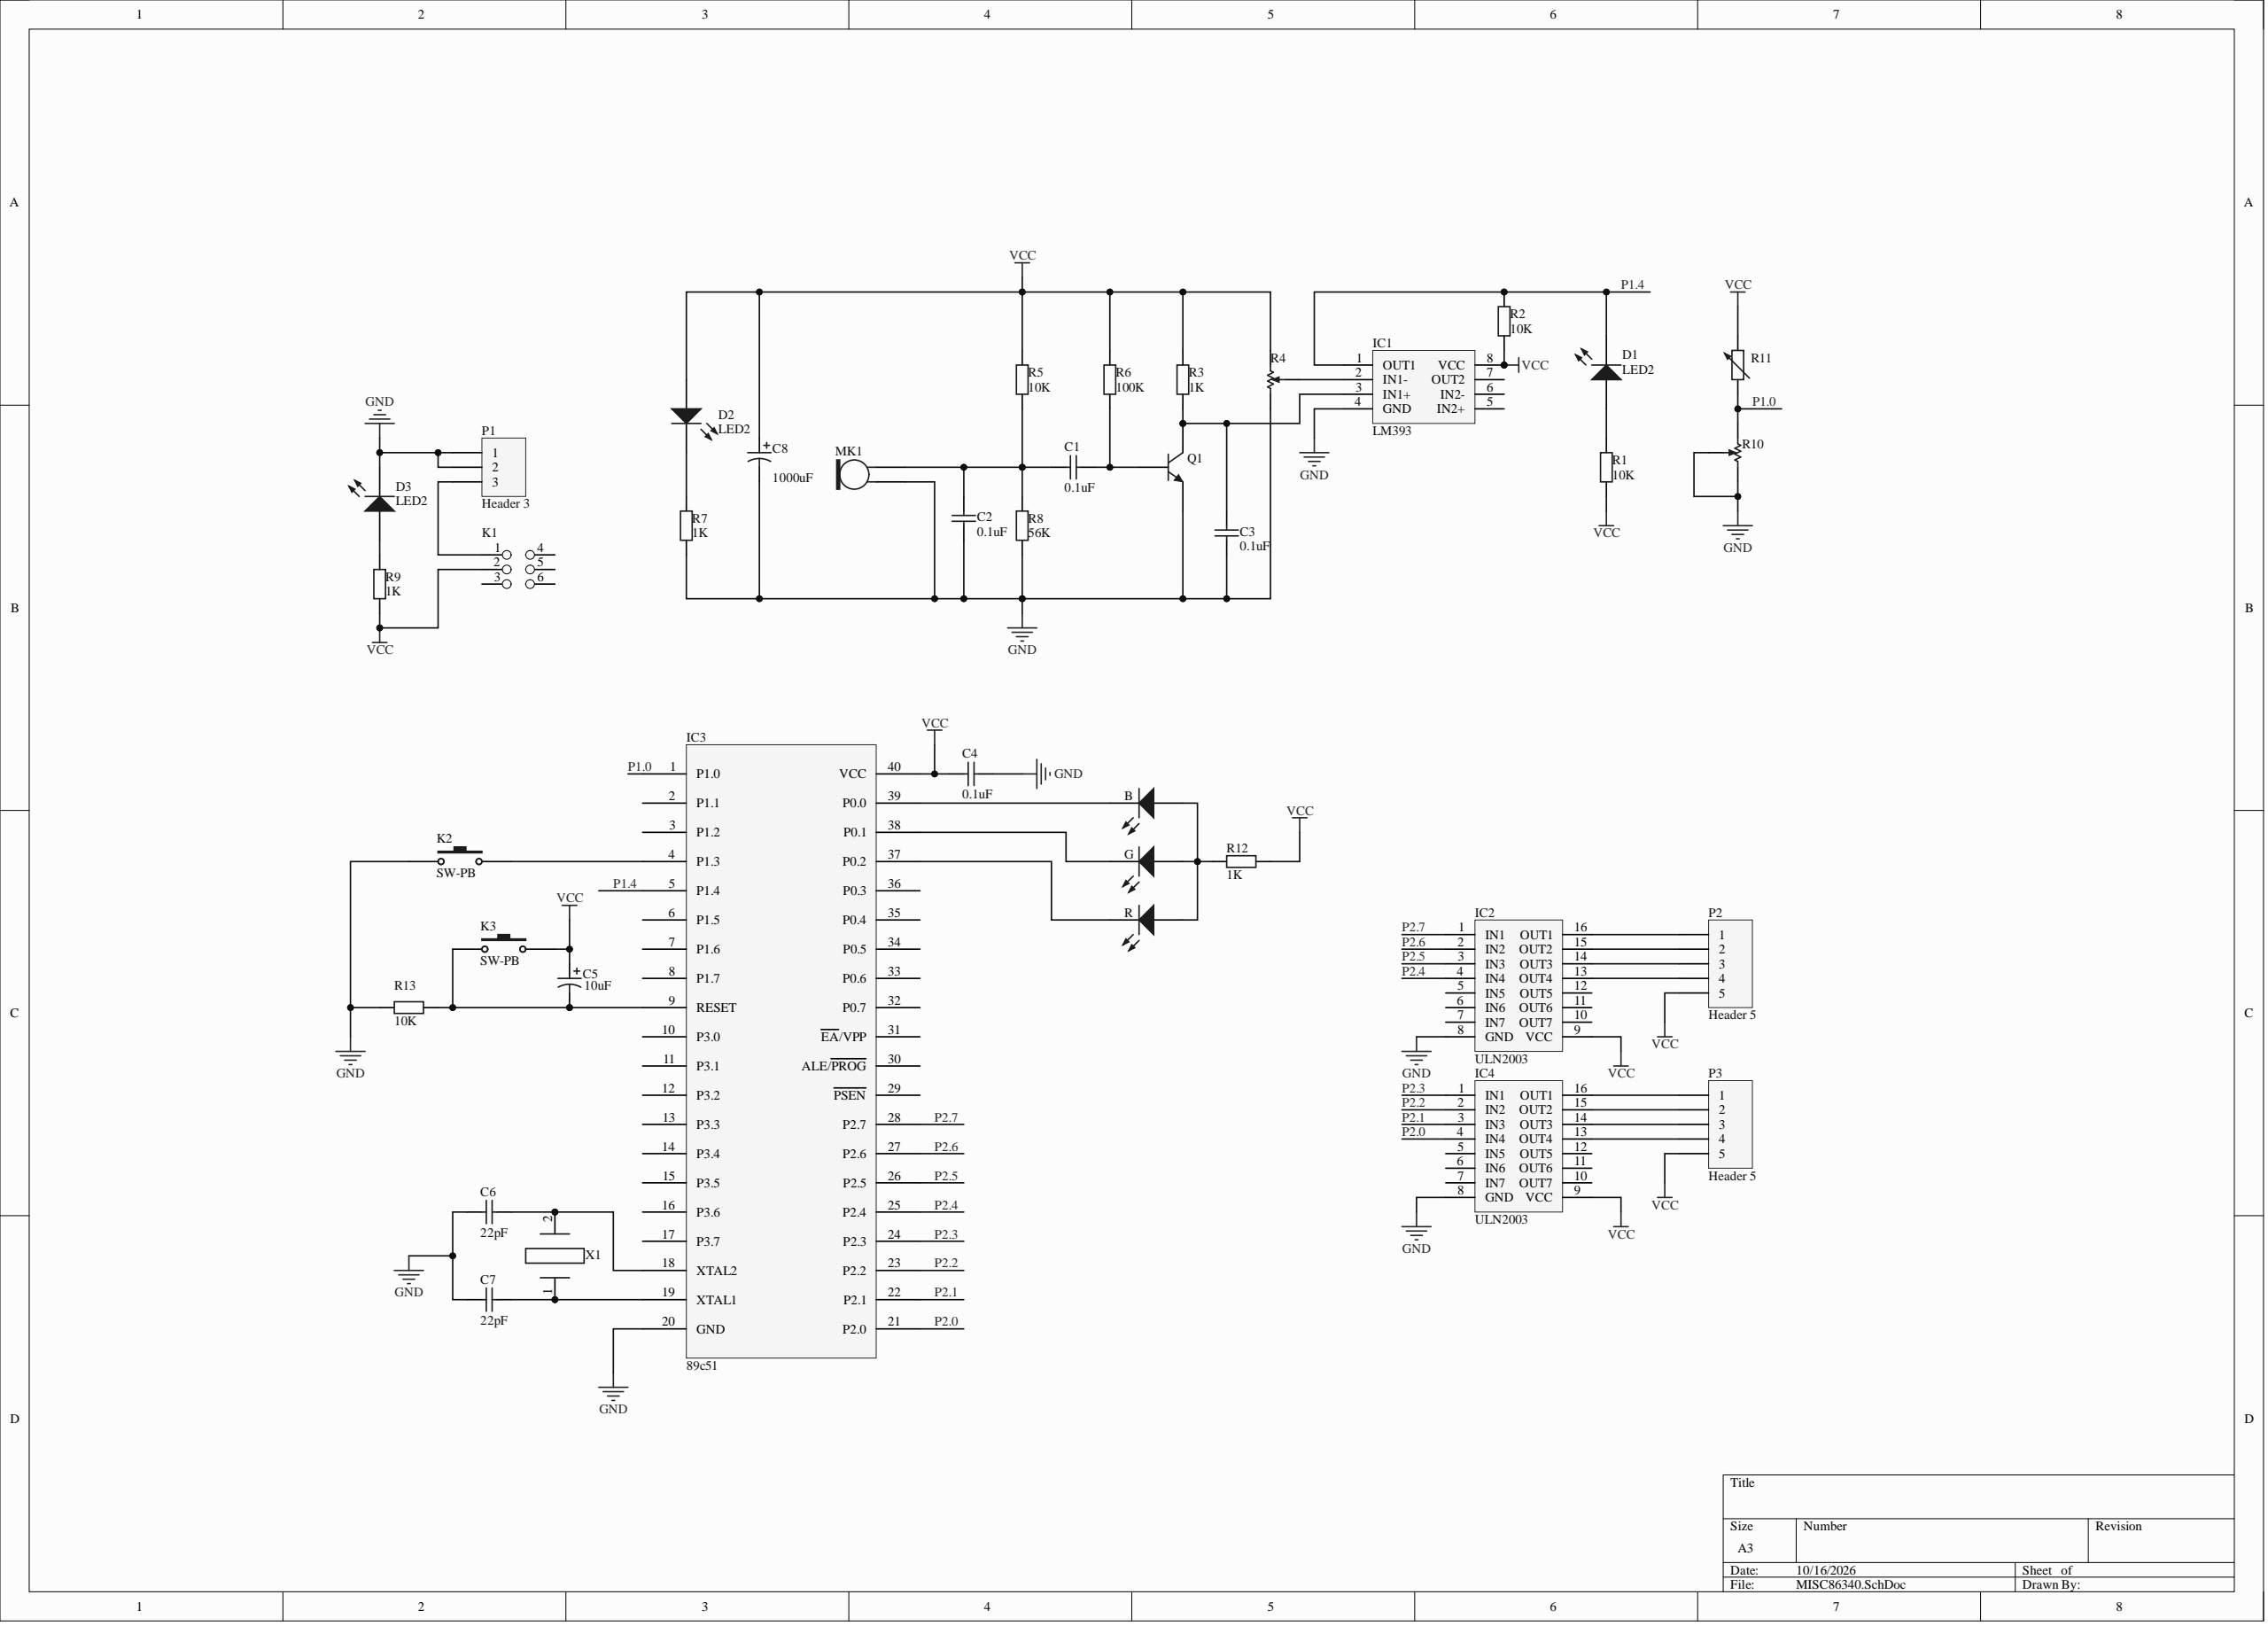Circuit board | Altium Designer | 40 parts | 36 nets
Bill of materials:
Comment,Description,Designator,Footprint,LibRef,Quantity
"LED2","Typical RED, GREEN, YELLOW, AMBER GaAs LED","B, D1, D2, D3, G, R","3.2X1.6X1.1","LED2","6"
"Cap","Capacitor","C1, C2, C3, C4, C6, C7","RAD-0.3","Cap","6"
"Cap Pol1","Polarized Capacitor (Radial)","C5, C8","RB7.6-15","Cap Pol1","2"
"LM393","","IC1","LM393","Component_1","1"
"ULN2003","","IC2, IC4","ULN2003","Component_1","2"
"89c51","","IC3","89c51","Component_1","1"
"Component_1","","K1","自锁开关","Component_1","1"
"SW-PB","Switch","K2, K3","SPST-2","SW-PB","2"
"Mic2","Microphone","MK1","PIN2","Mic2","1"
"Header 3","Header, 3-Pin","P1","HDR1X3","Header 3","1"
"Header 5","Header, 5-Pin","P2, P3","HDR1X5","Header 5","2"
"2N3904","NPN General Purpose Amplifier","Q1","TO-92A","2N3904","1"
"Res2","Resistor","R1, R2, R3, R5, R6, R12, R13","AXIAL-0.4","Res2","7"
"RPot SM","Square Trimming Potentiometer","R4, R10","POT4MM-2","RPot SM","2"
"1K","Resistor","R7, R9","AXIAL-0.4","Res2","2"
"56K","Resistor","R8","AXIAL-0.4","Res2","1"
"Res Adj2","Variable Resistor","R11","AXIAL-0.6","Res Adj2","1"
"Component_1","","X1","LC-HC-49S","Component_1","1"
Netlist (Protel format):
[
B
3.2X1.6X1.1
LED2



]
[
C1
RAD-0.3
Cap



]
[
C2
RAD-0.3
Cap



]
[
C3
RAD-0.3
Cap



]
[
C4
RAD-0.3
Cap



]
[
C5
RB7.6-15
Cap Pol1



]
[
C6
RAD-0.3
Cap



]
[
C7
RAD-0.3
Cap



]
[
C8
RB7.6-15
Cap Pol1



]
[
D1
3.2X1.6X1.1
LED2



]
[
D2
3.2X1.6X1.1
LED2



]
[
D3
3.2X1.6X1.1
LED2



]
[
G
3.2X1.6X1.1
LED2



]
[
IC1
LM393
LM393



]
[
IC2
ULN2003
ULN2003



]
[
IC3
89c51
89c51



]
[
IC4
ULN2003
ULN2003



]
[
K1
自锁开关
Component_1



]
[
K2
SPST-2
SW-PB



]
[
K3
SPST-2
SW-PB



]
[
MK1
PIN2
Mic2



]
[
P1
HDR1X3
Header 3



]
[
P2
HDR1X5
Header 5



]
[
P3
HDR1X5
Header 5



]
[
Q1
TO-92A
2N3904



]
[
R
3.2X1.6X1.1
LED2



]
[
R1
AXIAL-0.4
Res2



]
[
R2
AXIAL-0.4
Res2



]
[
R3
AXIAL-0.4
Res2



]
[
R4
POT4MM-2
RPot SM



]
[
R5
AXIAL-0.4
Res2



]
[
R6
AXIAL-0.4
Res2



]
[
R7
AXIAL-0.4
1K



]
[
R8
AXIAL-0.4
56K



]
[
R9
AXIAL-0.4
1K



]
[
R10
POT4MM-2
RPot SM



]
[
R11
AXIAL-0.6
Res Adj2



]
[
R12
AXIAL-0.4
Res2



]
[
R13
AXIAL-0.4
Res2



]
[
X1
LC-HC-49S
Component_1



]
(
VCC
C4-1
C5-1
C8-1
D2-1
IC1-8
IC2-9
IC3-40
IC4-9
K1-2
K3-2
P2-5
P3-5
R1-1
R2-1
R3-2
R4-CW
R5-2
R6-2
R9-1
R11-2
R12-1
)
(
P2.7
IC2-1
IC3-28
)
(
P2.6
IC2-2
IC3-27
)
(
P2.5
IC2-3
IC3-26
)
(
P2.4
IC2-4
IC3-25
)
(
P2.3
IC3-24
IC4-1
)
(
P2.2
IC3-23
IC4-2
)
(
P2.1
IC3-22
IC4-3
)
(
P2.0
IC3-21
IC4-4
)
(
P1.4
D1-2
IC1-1
IC3-5
R2-2
)
(
P1.0
IC3-1
R10-CCW
R11-1
)
(
NetK1_1
K1-1
P1-3
)
(
NetIC4_16
IC4-16
P3-1
)
(
NetIC4_15
IC4-15
P3-2
)
(
NetIC4_14
IC4-14
P3-3
)
(
NetIC4_13
IC4-13
P3-4
)
(
NetIC3_37
IC3-37
R-2
)
(
NetIC3_4
IC3-4
K2-2
)
(
NetIC2_16
IC2-16
P2-1
)
(
NetIC2_15
IC2-15
P2-2
)
(
NetIC2_14
IC2-14
P2-3
)
(
NetIC2_13
IC2-13
P2-4
)
(
NetIC1_2
IC1-2
R4-W
)
(
NetG_2
G-2
IC3-38
)
(
NetD3_1
D3-1
R9-2
)
(
NetD2_2
D2-2
R7-2
)
(
NetD1_1
D1-1
R1-2
)
(
NetC7_1
C7-1
IC3-19
X1-1
)
(
NetC6_1
C6-1
IC3-18
X1-2
)
(
NetC5_2
C5-2
IC3-9
K3-1
R13-1
)
(
NetC3_1
C3-1
IC1-3
Q1-3
R3-1
)
(
NetC1_2
C1-2
Q1-2
R6-1
)
(
NetC1_1
C1-1
C2-1
MK1-2
R5-1
R8-2
)
(
NetB_2
B-2
IC3-39
)
(
NetB_1
B-1
G-1
R-1
R12-2
)
(
GND
C2-2
C3-2
C4-2
C6-2
C7-2
C8-2
D3-2
IC1-4
IC2-8
IC3-20
IC4-8
K2-1
MK1-1
P1-1
P1-2
Q1-1
R4-CCW
R7-1
R8-1
R10-CW
R10-W
R13-2
)